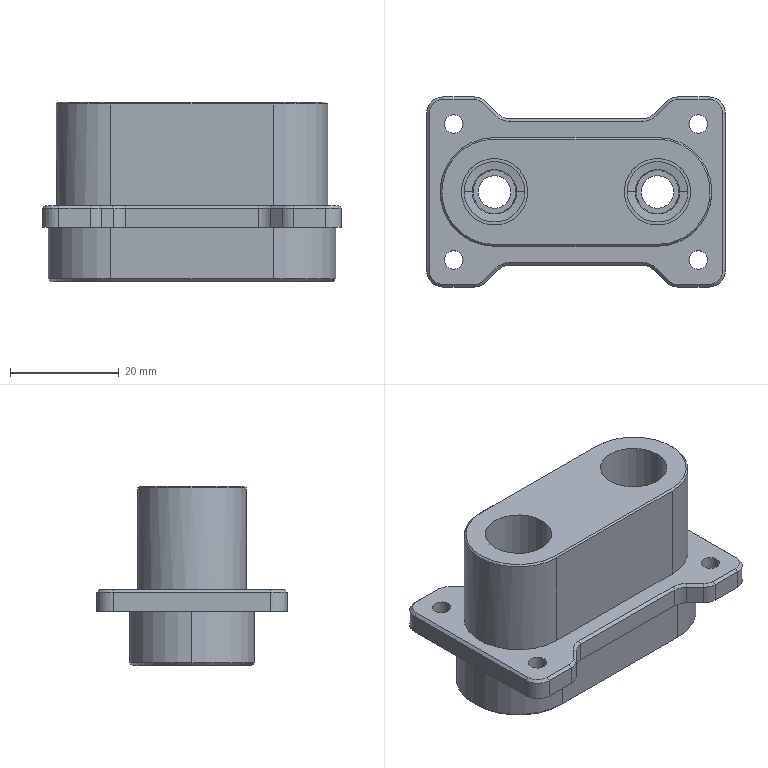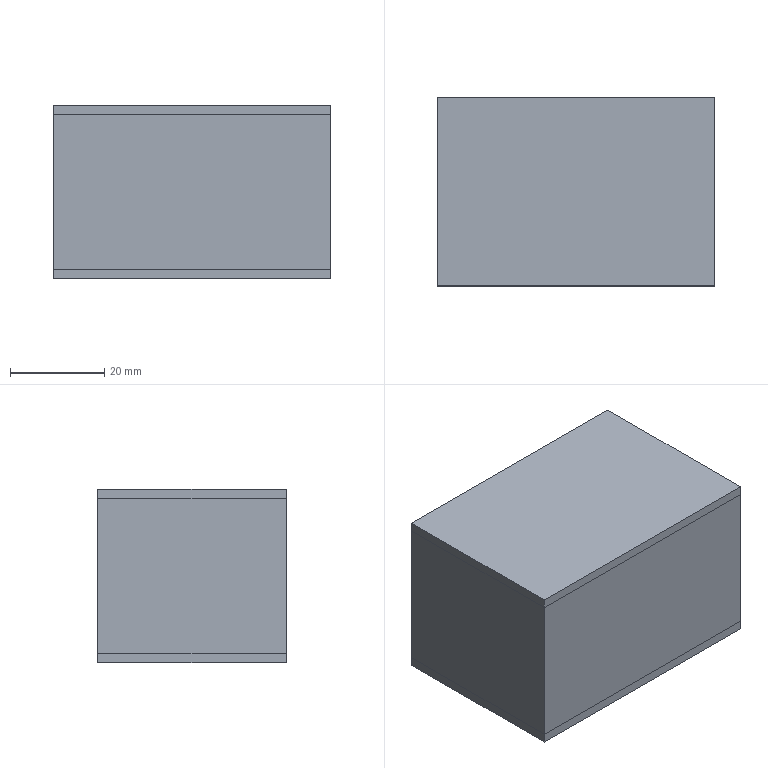CAM job | NX | 3-axis milling, drilling | part box 55 x 35 x 33 mm | stock box 59 x 40 x 37 mm
Tools:
number,name,description,diameter,corner_radius,flute_length,length,flutes
3,D6点钻,定心钻D6,6.0,0.0,57.0,93.0,2
9,D4开粗,D4,4.0,0.0,12.0,50.0,2
11,D4精光,D4,4.0,0.0,12.0,50.0,2
2,D6开粗,D6,6.0,0.0,16.0,60.0,2
6,D6精光,D6,6.0,0.0,16.0,60.0,2
1,D50面刀,Milling Tool-5 Parameters,50.0,0.0,50.0,75.0,2
4,D11.7钻头,Drilling Tool,11.7,0.0,35.0,50.0,2
5,G4-1,Thread Mill,9.7,0.0,30.0,50.0,2
7,D6.5钻头,Drilling Tool,6.5,0.0,35.0,50.0,2
10,D7.9成型刀,Milling Tool-5 Parameters,7.9,1.0,30.0,30.0,4
8,D3.4钻头,Drilling Tool,3.4,0.0,35.0,50.0,2
Operations:
program,operation,operation_type,tool,method,geometry_group,spindle_rpm,surface_speed,feed_per_tooth,feed_cut,feed_plunge,cut_length_mm,path_length_mm,cut_time_min,machine_time_min
XX-CNC1,PLANAR_MILL,PlanarMilling,D50面刀,METHOD,MCS_1,3500.0,100.0,0.1178,800.0,100.0,123.0,179.0,0.1538,0.1594
XX-CNC1,ADAPTIVE_MILLING,CavityMilling,D6开粗,METHOD,W1,5500.0,100.0,0.1178,2500.0,100.0,3895.575,4246.331,1.162,1.197
XX-CNC1,DRILLING,Operation,D6点钻,METHOD,W1,3000.0,0.0,0.0,200.0,0.0,9.0,111.15,0.045,0.0552
XX-CNC1,DRILLING_1,Operation,D6点钻,METHOD,W1,3000.0,0.0,0.0,200.0,0.0,18.8,222.059,0.094,0.1143
XX-CNC1,DRILLING_1_COPY,Operation,D3.4钻头,METHOD,W1,3000.0,0.0,0.0,200.0,0.0,44.0,272.459,0.22,0.2428
XX-CNC1,DRILLING_COPY,Operation,D11.7钻头,METHOD,W1,2500.0,0.0,0.0,200.0,0.0,41.03,175.21,0.2052,0.2186
XX-CNC1,DRILLING_COPY_COPY,Operation,D6.5钻头,METHOD,W1,2500.0,0.0,0.0,200.0,0.0,56.0,205.15,0.28,0.2949
XX-CNC1,PLANAR_MILL_1,PlanarMilling,D6点钻,METHOD,W1,3500.0,100.0,0.1178,1000.0,100.0,151.965,211.965,0.152,0.158
XX-CNC1,PLANAR_MILL_1_COPY,PlanarMilling,D6点钻,METHOD,W1,3500.0,100.0,0.1178,1000.0,100.0,82.126,232.392,0.0821,0.0972
XX-CNC1,PLANAR_MILL_1_COPY_1,PlanarMilling,D6点钻,METHOD,W1,3500.0,100.0,0.1178,1000.0,100.0,206.435,287.435,0.2064,0.2145
XX-CNC1,PLANAR_MILL_2,PlanarMilling,D6精光,METHOD,W1,4500.0,84.0,0.0889,800.0,100.0,351.029,427.029,0.4388,0.4464
XX-CNC1,PLANAR_MILL_2_COPY,PlanarMilling,D6精光,METHOD,W1,4500.0,84.0,0.0889,800.0,100.0,161.789,237.789,0.2022,0.2098
XX-CNC1,PLANAR_MILL_1_COPY_1_COPY,PlanarMilling,D6精光,METHOD,W1,3500.0,100.0,0.1178,800.0,100.0,419.885,507.885,0.5249,0.5337
XX-CNC1,THREAD_MILLING,ThreadMilling,G4-1,METHOD,W1,4000.0,0.0,0.0,200.0,100.0,169.444,386.786,0.8472,0.869
XX-CNC2,ADAPTIVE_MILLING_COPY,CavityMilling,D6开粗,METHOD,W2,5500.0,100.0,0.1178,2500.0,100.0,6928.13,7298.94,2.195,2.232
XX-CNC2,PLANAR_MILL_3,PlanarMilling,D50面刀,METHOD,MCS_2,3500.0,100.0,0.1178,800.0,100.0,113.0,169.0,0.1412,0.1468
XX-CNC2,DRILLING_2,Operation,D6点钻,METHOD,MCS_2,3000.0,0.0,0.0,200.0,0.0,9.0,111.15,0.045,0.0552
XX-CNC2,DRILLING_2_COPY,Operation,D6.5钻头,METHOD,MCS_2,3000.0,0.0,0.0,200.0,0.0,50.0,193.15,0.25,0.2643
XX-CNC2,ADAPTIVE_MILLING_1,CavityMilling,D4开粗,METHOD,W2,4500.0,100.0,0.1178,600.0,100.0,1509.667,2573.259,2.509,2.615
XX-CNC2,DRILLING_2_COPY_COPY,Operation,D7.9成型刀,METHOD,MCS_2,4000.0,0.0,0.0,80.0,0.0,37.5,168.15,0.4688,0.4818
XX-CNC2,PLANAR_MILL_5,PlanarMilling,D6点钻,METHOD,W2,3500.0,100.0,0.1178,800.0,100.0,140.655,199.655,0.1758,0.1817
XX-CNC2,PLANAR_MILL_5_COPY,PlanarMilling,D6点钻,METHOD,W2,3500.0,100.0,0.1178,800.0,100.0,200.152,298.152,0.2502,0.26
XX-CNC2,DRILLING_3,Operation,D6点钻,METHOD,W2,3000.0,56.0,0.0333,200.0,0.0,18.8,259.979,0.094,0.1181
XX-CNC2,PLANAR_MILL_7,PlanarMilling,D6精光,METHOD,MCS_2,5500.0,103.0,0.0727,800.0,100.0,336.186,430.186,0.4202,0.4296
XX-CNC2,PLANAR_MILL_7_COPY,PlanarMilling,D6精光,METHOD,MCS_2,5500.0,103.0,0.0727,800.0,100.0,156.246,250.246,0.1953,0.2047
XX-CNC2,PLANAR_MILL_4,PlanarMilling,D4精光,METHOD,W2,5500.0,100.0,0.1178,200.0,100.0,78.03,261.067,0.3902,0.4085
XX-CNC2,PLANAR_MILL_4_COPY,PlanarMilling,D4精光,METHOD,W2,5500.0,100.0,0.1178,200.0,100.0,69.374,260.225,0.3469,0.366
XX-CNC5,PLANAR_MILL_6,PlanarMilling,D6开粗,METHOD,MCS_5,6500.0,122.0,0.1538,2000.0,100.0,4769.79,5954.836,2.385,2.503
XX-CNC5,PLANAR_MILL_6_COPY,PlanarMilling,D6开粗,METHOD,MCS_5,6500.0,122.0,0.0615,800.0,100.0,288.618,362.618,0.3608,0.3682
XX-CNC5,PLANAR_MILL_6_COPY_COPY,PlanarMilling,D6开粗,METHOD,MCS_5,6500.0,122.0,0.0615,800.0,100.0,120.949,192.949,0.1512,0.1584